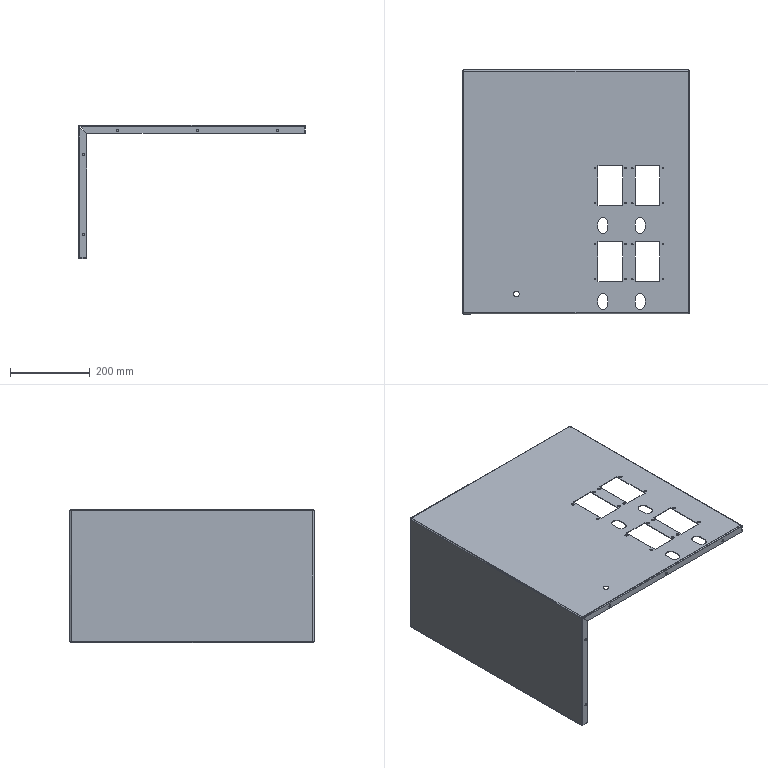Part | SolidWorks | features LPattern 4, ICE 3, Cut 2, EdgeFlange 2, 3DProfileFeature 1, FlatPattern 1, HoleWzd 1, SMBaseFlange 1, SheetMetal 1 | 1 solid | 186 faces | box 568 x 611 x 333 mm | volume 859533 mm3 | cylinder 98 | plane 76 | spline 12 | commonest cylinder face diameters 3.3 x32 8 x32 6 x17 25 x8 3 x7 14 x2